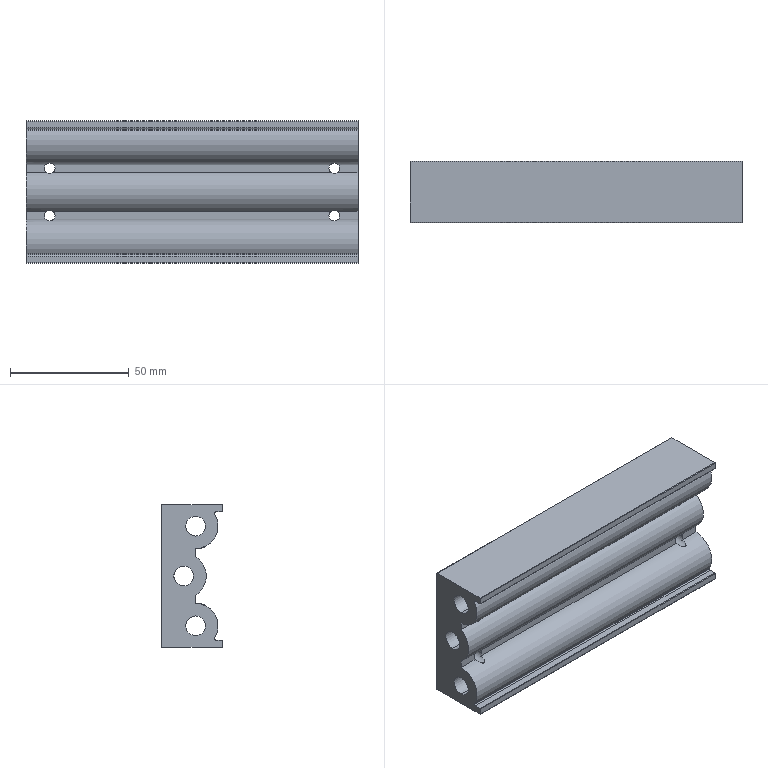Part | NX | 1 solid | 247 faces | box 140 x 26 x 60 mm | volume 146568 mm3 | plane 124 | cylinder 95 | cone 28 | commonest cylinder face diameters 4 x42 2.5 x28 4.5 x8 0.4 x6 8.3 x6 19 x3